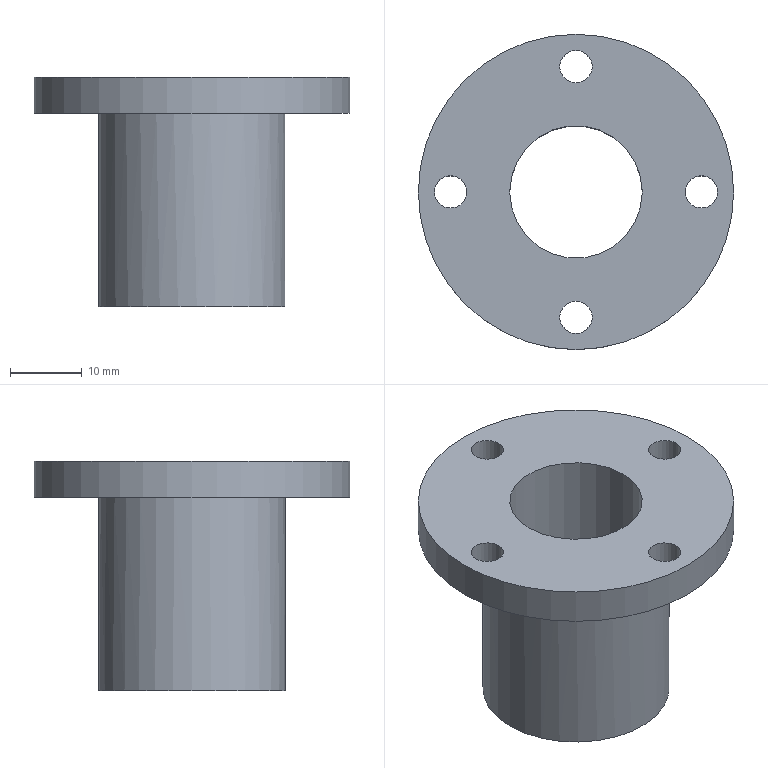Part | STEP file | YBQDJ-YL-17 | 1 solid | 10 faces | box 44 x 44 x 32 mm | volume 13018 mm3 | cylinder 7 | plane 3 | commonest cylinder face diameters 4.5 x4 18.5 x1 26 x1 44 x1
STEP:
#1=CARTESIAN_POINT('',(0.,0.,0.));
#2=DIRECTION('',(0.,0.,1.));
#3=DIRECTION('',(1.,0.,0.));
#4=AXIS2_PLACEMENT_3D('',#1,#2,#3);
#5=CARTESIAN_POINT('',(306.5,-210.25,170.));
#6=VERTEX_POINT('',#5);
#7=CARTESIAN_POINT('',(306.5,-212.5,170.));
#8=DIRECTION('',(0.,0.,-1.));
#9=DIRECTION('',(0.,1.,0.));
#10=AXIS2_PLACEMENT_3D('',#7,#8,#9);
#11=CIRCLE('',#10,2.25);
#12=CARTESIAN_POINT('',(306.5,-212.5,170.));
#13=DIRECTION('',(0.,0.,-1.));
#14=DIRECTION('',(1.,0.,0.));
#15=AXIS2_PLACEMENT_3D('',#12,#13,#14);
#16=CYLINDRICAL_SURFACE('',#15,2.25);
#17=CARTESIAN_POINT('',(4.712,0.));
#18=DIRECTION('',(1.,0.));
#19=VECTOR('',#18,1.);
#20=LINE('',#17,#19);
#21=(GEOMETRIC_REPRESENTATION_CONTEXT(2)PARAMETRIC_REPRESENTATION_CONTEXT()REPRESENTATION_CONTEXT('',''));
#22=DEFINITIONAL_REPRESENTATION('',(#20),#21);
#23=PCURVE('',#16,#22);
#24=CARTESIAN_POINT('',(306.5,-195.,170.));
#25=DIRECTION('',(0.,0.,1.));
#26=DIRECTION('',(0.,-1.,0.));
#27=AXIS2_PLACEMENT_3D('',#24,#25,#26);
#28=PLANE('',#27);
#29=CARTESIAN_POINT('',(15.25,0.));
#30=CARTESIAN_POINT('',(15.25,3.897));
#31=CARTESIAN_POINT('',(18.625,1.949));
#32=CARTESIAN_POINT('',(22.,0.));
#33=CARTESIAN_POINT('',(18.625,-1.949));
#34=CARTESIAN_POINT('',(15.25,-3.897));
#35=CARTESIAN_POINT('',(15.25,0.));
#36=(BOUNDED_CURVE()B_SPLINE_CURVE(2,(#29,#30,#31,#32,#33,#34,#35),.UNSPECIFIED.,.T.,.F.)B_SPLINE_CURVE_WITH_KNOTS((1,2,2,2,2,1),(-2.094,0.,2.094,4.189,6.283,8.378),.UNSPECIFIED.)CURVE()GEOMETRIC_REPRESENTATION_ITEM()RATIONAL_B_SPLINE_CURVE((1.,0.5,1.,0.5,1.,0.5,1.))REPRESENTATION_ITEM(''));
#37=(GEOMETRIC_REPRESENTATION_CONTEXT(2)PARAMETRIC_REPRESENTATION_CONTEXT()REPRESENTATION_CONTEXT('',''));
#38=DEFINITIONAL_REPRESENTATION('',(#36),#37);
#39=PCURVE('',#28,#38);
#40=SURFACE_CURVE('',#11,(#23,#39),.PCURVE_S1.);
#41=EDGE_CURVE('',#6,#6,#40,.T.);
#42=ORIENTED_EDGE('',*,*,#41,.T.);
#43=CARTESIAN_POINT('',(306.5,-210.25,165.));
#44=VERTEX_POINT('',#43);
#45=CARTESIAN_POINT('',(306.5,-210.25,170.));
#46=CARTESIAN_POINT('',(306.5,-210.25,165.));
#47=B_SPLINE_CURVE_WITH_KNOTS('',1,(#45,#46),.UNSPECIFIED.,.F.,.F.,(2,2),(0.,5.),.PIECEWISE_BEZIER_KNOTS.);
#48=CARTESIAN_POINT('',(10.996,0.));
#49=DIRECTION('',(0.,1.));
#50=VECTOR('',#49,1.);
#51=LINE('',#48,#50);
#52=(GEOMETRIC_REPRESENTATION_CONTEXT(2)PARAMETRIC_REPRESENTATION_CONTEXT()REPRESENTATION_CONTEXT('',''));
#53=DEFINITIONAL_REPRESENTATION('',(#51),#52);
#54=PCURVE('',#16,#53);
#55=CARTESIAN_POINT('',(4.712,0.));
#56=DIRECTION('',(0.,1.));
#57=VECTOR('',#56,1.);
#58=LINE('',#55,#57);
#59=(GEOMETRIC_REPRESENTATION_CONTEXT(2)PARAMETRIC_REPRESENTATION_CONTEXT()REPRESENTATION_CONTEXT('',''));
#60=DEFINITIONAL_REPRESENTATION('',(#58),#59);
#61=PCURVE('',#16,#60);
#62=SEAM_CURVE('',#47,(#54,#61),.PCURVE_S1.);
#63=EDGE_CURVE('',#6,#44,#62,.T.);
#64=ORIENTED_EDGE('',*,*,#63,.T.);
#65=CARTESIAN_POINT('',(306.5,-212.5,165.));
#66=DIRECTION('',(0.,0.,1.));
#67=DIRECTION('',(0.,1.,0.));
#68=AXIS2_PLACEMENT_3D('',#65,#66,#67);
#69=CIRCLE('',#68,2.25);
#70=CARTESIAN_POINT('',(10.996,5.));
#71=DIRECTION('',(-1.,0.));
#72=VECTOR('',#71,1.);
#73=LINE('',#70,#72);
#74=(GEOMETRIC_REPRESENTATION_CONTEXT(2)PARAMETRIC_REPRESENTATION_CONTEXT()REPRESENTATION_CONTEXT('',''));
#75=DEFINITIONAL_REPRESENTATION('',(#73),#74);
#76=PCURVE('',#16,#75);
#77=CARTESIAN_POINT('',(306.5,-195.,165.));
#78=DIRECTION('',(0.,0.,1.));
#79=DIRECTION('',(0.,-1.,0.));
#80=AXIS2_PLACEMENT_3D('',#77,#78,#79);
#81=PLANE('',#80);
#82=CARTESIAN_POINT('',(17.5,0.));
#83=DIRECTION('',(-1.,0.));
#84=AXIS2_PLACEMENT_2D('',#82,#83);
#85=CIRCLE('',#84,2.25);
#86=(GEOMETRIC_REPRESENTATION_CONTEXT(2)PARAMETRIC_REPRESENTATION_CONTEXT()REPRESENTATION_CONTEXT('',''));
#87=DEFINITIONAL_REPRESENTATION('',(#85),#86);
#88=PCURVE('',#81,#87);
#89=SURFACE_CURVE('',#69,(#76,#88),.PCURVE_S1.);
#90=EDGE_CURVE('',#44,#44,#89,.T.);
#91=ORIENTED_EDGE('',*,*,#90,.T.);
#92=ORIENTED_EDGE('',*,*,#63,.F.);
#93=EDGE_LOOP('',(#42,#64,#91,#92));
#94=FACE_BOUND('',#93,.F.);
#95=ADVANCED_FACE('',(#94),#16,.F.);
#96=CARTESIAN_POINT('',(297.25,-195.,138.));
#97=VERTEX_POINT('',#96);
#98=CARTESIAN_POINT('',(315.75,-195.,138.));
#99=VERTEX_POINT('',#98);
#100=CARTESIAN_POINT('',(306.5,-195.,138.));
#101=DIRECTION('',(0.,0.,1.));
#102=DIRECTION('',(-1.,0.,0.));
#103=AXIS2_PLACEMENT_3D('',#100,#101,#102);
#104=CIRCLE('',#103,9.25);
#105=CARTESIAN_POINT('',(306.5,-195.,138.));
#106=DIRECTION('',(0.,0.,-1.));
#107=DIRECTION('',(0.,1.,0.));
#108=AXIS2_PLACEMENT_3D('',#105,#106,#107);
#109=PLANE('',#108);
#110=CARTESIAN_POINT('',(0.,-9.25));
#111=CARTESIAN_POINT('',(-16.021,-9.25));
#112=CARTESIAN_POINT('',(-8.011,4.625));
#113=CARTESIAN_POINT('',(0.,18.5));
#114=CARTESIAN_POINT('',(8.011,4.625));
#115=CARTESIAN_POINT('',(16.021,-9.25));
#116=CARTESIAN_POINT('',(0.,-9.25));
#117=(BOUNDED_CURVE()B_SPLINE_CURVE(2,(#110,#111,#112,#113,#114,#115,#116),.UNSPECIFIED.,.T.,.F.)B_SPLINE_CURVE_WITH_KNOTS((1,2,2,2,2,1),(-2.094,0.,2.094,4.189,6.283,8.378),.UNSPECIFIED.)CURVE()GEOMETRIC_REPRESENTATION_ITEM()RATIONAL_B_SPLINE_CURVE((1.,0.5,1.,0.5,1.,0.5,1.))REPRESENTATION_ITEM(''));
#118=(GEOMETRIC_REPRESENTATION_CONTEXT(2)PARAMETRIC_REPRESENTATION_CONTEXT()REPRESENTATION_CONTEXT('',''));
#119=DEFINITIONAL_REPRESENTATION('',(#117),#118);
#120=PCURVE('',#109,#119);
#121=CARTESIAN_POINT('',(306.5,-195.,142.));
#122=DIRECTION('',(0.,0.,1.));
#123=DIRECTION('',(0.,-1.,0.));
#124=AXIS2_PLACEMENT_3D('',#121,#122,#123);
#125=CYLINDRICAL_SURFACE('',#124,9.25);
#126=CARTESIAN_POINT('',(4.712,-4.));
#127=DIRECTION('',(1.,0.));
#128=VECTOR('',#127,1.);
#129=LINE('',#126,#128);
#130=(GEOMETRIC_REPRESENTATION_CONTEXT(2)PARAMETRIC_REPRESENTATION_CONTEXT()REPRESENTATION_CONTEXT('',''));
#131=DEFINITIONAL_REPRESENTATION('',(#129),#130);
#132=PCURVE('',#125,#131);
#133=SURFACE_CURVE('',#104,(#120,#132),.PCURVE_S1.);
#134=EDGE_CURVE('',#97,#99,#133,.T.);
#135=ORIENTED_EDGE('',*,*,#134,.T.);
#136=CARTESIAN_POINT('',(306.5,-195.,138.));
#137=DIRECTION('',(0.,0.,1.));
#138=DIRECTION('',(-1.,0.,0.));
#139=AXIS2_PLACEMENT_3D('',#136,#137,#138);
#140=CIRCLE('',#139,9.25);
#141=CARTESIAN_POINT('',(0.,-9.25));
#142=CARTESIAN_POINT('',(-16.021,-9.25));
#143=CARTESIAN_POINT('',(-8.011,4.625));
#144=CARTESIAN_POINT('',(0.,18.5));
#145=CARTESIAN_POINT('',(8.011,4.625));
#146=CARTESIAN_POINT('',(16.021,-9.25));
#147=CARTESIAN_POINT('',(0.,-9.25));
#148=(BOUNDED_CURVE()B_SPLINE_CURVE(2,(#141,#142,#143,#144,#145,#146,#147),.UNSPECIFIED.,.T.,.F.)B_SPLINE_CURVE_WITH_KNOTS((1,2,2,2,2,1),(-2.094,0.,2.094,4.189,6.283,8.378),.UNSPECIFIED.)CURVE()GEOMETRIC_REPRESENTATION_ITEM()RATIONAL_B_SPLINE_CURVE((1.,0.5,1.,0.5,1.,0.5,1.))REPRESENTATION_ITEM(''));
#149=(GEOMETRIC_REPRESENTATION_CONTEXT(2)PARAMETRIC_REPRESENTATION_CONTEXT()REPRESENTATION_CONTEXT('',''));
#150=DEFINITIONAL_REPRESENTATION('',(#148),#149);
#151=PCURVE('',#109,#150);
#152=CARTESIAN_POINT('',(-1.571,-4.));
#153=DIRECTION('',(1.,0.));
#154=VECTOR('',#153,1.);
#155=LINE('',#152,#154);
#156=(GEOMETRIC_REPRESENTATION_CONTEXT(2)PARAMETRIC_REPRESENTATION_CONTEXT()REPRESENTATION_CONTEXT('',''));
#157=DEFINITIONAL_REPRESENTATION('',(#155),#156);
#158=PCURVE('',#125,#157);
#159=SURFACE_CURVE('',#140,(#151,#158),.PCURVE_S1.);
#160=EDGE_CURVE('',#99,#97,#159,.T.);
#161=ORIENTED_EDGE('',*,*,#160,.T.);
#162=EDGE_LOOP('',(#135,#161));
#163=FACE_BOUND('',#162,.T.);
#164=CARTESIAN_POINT('',(293.5,-195.,138.));
#165=VERTEX_POINT('',#164);
#166=CARTESIAN_POINT('',(306.5,-195.,138.));
#167=DIRECTION('',(0.,0.,-1.));
#168=DIRECTION('',(-1.,0.,0.));
#169=AXIS2_PLACEMENT_3D('',#166,#167,#168);
#170=CIRCLE('',#169,13.);
#171=CARTESIAN_POINT('',(0.,0.));
#172=DIRECTION('',(0.,-1.));
#173=AXIS2_PLACEMENT_2D('',#171,#172);
#174=CIRCLE('',#173,13.);
#175=(GEOMETRIC_REPRESENTATION_CONTEXT(2)PARAMETRIC_REPRESENTATION_CONTEXT()REPRESENTATION_CONTEXT('',''));
#176=DEFINITIONAL_REPRESENTATION('',(#174),#175);
#177=PCURVE('',#109,#176);
#178=CARTESIAN_POINT('',(306.5,-195.,165.));
#179=DIRECTION('',(0.,0.,-1.));
#180=DIRECTION('',(0.,1.,0.));
#181=AXIS2_PLACEMENT_3D('',#178,#179,#180);
#182=CYLINDRICAL_SURFACE('',#181,13.);
#183=CARTESIAN_POINT('',(4.712,27.));
#184=DIRECTION('',(1.,0.));
#185=VECTOR('',#184,1.);
#186=LINE('',#183,#185);
#187=(GEOMETRIC_REPRESENTATION_CONTEXT(2)PARAMETRIC_REPRESENTATION_CONTEXT()REPRESENTATION_CONTEXT('',''));
#188=DEFINITIONAL_REPRESENTATION('',(#186),#187);
#189=PCURVE('',#182,#188);
#190=SURFACE_CURVE('',#170,(#177,#189),.PCURVE_S1.);
#191=EDGE_CURVE('',#165,#165,#190,.T.);
#192=ORIENTED_EDGE('',*,*,#191,.T.);
#193=EDGE_LOOP('',(#192));
#194=FACE_BOUND('',#193,.T.);
#195=ADVANCED_FACE('',(#163,#194),#109,.T.);
#196=CARTESIAN_POINT('',(291.25,-195.,170.));
#197=VERTEX_POINT('',#196);
#198=CARTESIAN_POINT('',(289.,-195.,170.));
#199=DIRECTION('',(0.,0.,1.));
#200=DIRECTION('',(1.,0.,0.));
#201=AXIS2_PLACEMENT_3D('',#198,#199,#200);
#202=CIRCLE('',#201,2.25);
#203=CARTESIAN_POINT('',(289.,-195.,170.));
#204=DIRECTION('',(0.,0.,-1.));
#205=DIRECTION('',(0.,1.,0.));
#206=AXIS2_PLACEMENT_3D('',#203,#204,#205);
#207=CYLINDRICAL_SURFACE('',#206,2.25);
#208=CARTESIAN_POINT('',(7.854,0.));
#209=DIRECTION('',(-1.,0.));
#210=VECTOR('',#209,1.);
#211=LINE('',#208,#210);
#212=(GEOMETRIC_REPRESENTATION_CONTEXT(2)PARAMETRIC_REPRESENTATION_CONTEXT()REPRESENTATION_CONTEXT('',''));
#213=DEFINITIONAL_REPRESENTATION('',(#211),#212);
#214=PCURVE('',#207,#213);
#215=CARTESIAN_POINT('',(0.,-17.5));
#216=DIRECTION('',(0.,1.));
#217=AXIS2_PLACEMENT_2D('',#215,#216);
#218=CIRCLE('',#217,2.25);
#219=(GEOMETRIC_REPRESENTATION_CONTEXT(2)PARAMETRIC_REPRESENTATION_CONTEXT()REPRESENTATION_CONTEXT('',''));
#220=DEFINITIONAL_REPRESENTATION('',(#218),#219);
#221=PCURVE('',#28,#220);
#222=SURFACE_CURVE('',#202,(#214,#221),.PCURVE_S1.);
#223=EDGE_CURVE('',#197,#197,#222,.T.);
#224=ORIENTED_EDGE('',*,*,#223,.F.);
#225=CARTESIAN_POINT('',(291.25,-195.,165.));
#226=VERTEX_POINT('',#225);
#227=CARTESIAN_POINT('',(291.25,-195.,170.));
#228=CARTESIAN_POINT('',(291.25,-195.,165.));
#229=B_SPLINE_CURVE_WITH_KNOTS('',1,(#227,#228),.UNSPECIFIED.,.F.,.F.,(2,2),(0.,5.),.PIECEWISE_BEZIER_KNOTS.);
#230=CARTESIAN_POINT('',(7.854,0.));
#231=DIRECTION('',(0.,1.));
#232=VECTOR('',#231,1.);
#233=LINE('',#230,#232);
#234=(GEOMETRIC_REPRESENTATION_CONTEXT(2)PARAMETRIC_REPRESENTATION_CONTEXT()REPRESENTATION_CONTEXT('',''));
#235=DEFINITIONAL_REPRESENTATION('',(#233),#234);
#236=PCURVE('',#207,#235);
#237=CARTESIAN_POINT('',(1.571,0.));
#238=DIRECTION('',(0.,1.));
#239=VECTOR('',#238,1.);
#240=LINE('',#237,#239);
#241=(GEOMETRIC_REPRESENTATION_CONTEXT(2)PARAMETRIC_REPRESENTATION_CONTEXT()REPRESENTATION_CONTEXT('',''));
#242=DEFINITIONAL_REPRESENTATION('',(#240),#241);
#243=PCURVE('',#207,#242);
#244=SEAM_CURVE('',#229,(#236,#243),.PCURVE_S1.);
#245=EDGE_CURVE('',#197,#226,#244,.T.);
#246=ORIENTED_EDGE('',*,*,#245,.T.);
#247=CARTESIAN_POINT('',(289.,-195.,165.));
#248=DIRECTION('',(0.,0.,1.));
#249=DIRECTION('',(1.,0.,0.));
#250=AXIS2_PLACEMENT_3D('',#247,#248,#249);
#251=CIRCLE('',#250,2.25);
#252=CARTESIAN_POINT('',(7.854,5.));
#253=DIRECTION('',(-1.,0.));
#254=VECTOR('',#253,1.);
#255=LINE('',#252,#254);
#256=(GEOMETRIC_REPRESENTATION_CONTEXT(2)PARAMETRIC_REPRESENTATION_CONTEXT()REPRESENTATION_CONTEXT('',''));
#257=DEFINITIONAL_REPRESENTATION('',(#255),#256);
#258=PCURVE('',#207,#257);
#259=CARTESIAN_POINT('',(0.,-17.5));
#260=DIRECTION('',(0.,1.));
#261=AXIS2_PLACEMENT_2D('',#259,#260);
#262=CIRCLE('',#261,2.25);
#263=(GEOMETRIC_REPRESENTATION_CONTEXT(2)PARAMETRIC_REPRESENTATION_CONTEXT()REPRESENTATION_CONTEXT('',''));
#264=DEFINITIONAL_REPRESENTATION('',(#262),#263);
#265=PCURVE('',#81,#264);
#266=SURFACE_CURVE('',#251,(#258,#265),.PCURVE_S1.);
#267=EDGE_CURVE('',#226,#226,#266,.T.);
#268=ORIENTED_EDGE('',*,*,#267,.T.);
#269=ORIENTED_EDGE('',*,*,#245,.F.);
#270=EDGE_LOOP('',(#224,#246,#268,#269));
#271=FACE_BOUND('',#270,.F.);
#272=ADVANCED_FACE('',(#271),#207,.F.);
#273=CARTESIAN_POINT('',(321.75,-195.,170.));
#274=VERTEX_POINT('',#273);
#275=CARTESIAN_POINT('',(324.,-195.,170.));
#276=DIRECTION('',(0.,0.,-1.));
#277=DIRECTION('',(-1.,0.,0.));
#278=AXIS2_PLACEMENT_3D('',#275,#276,#277);
#279=CIRCLE('',#278,2.25);
#280=CARTESIAN_POINT('',(324.,-195.,170.));
#281=DIRECTION('',(0.,0.,-1.));
#282=DIRECTION('',(0.,1.,0.));
#283=AXIS2_PLACEMENT_3D('',#280,#281,#282);
#284=CYLINDRICAL_SURFACE('',#283,2.25);
#285=CARTESIAN_POINT('',(4.712,0.));
#286=DIRECTION('',(1.,0.));
#287=VECTOR('',#286,1.);
#288=LINE('',#285,#287);
#289=(GEOMETRIC_REPRESENTATION_CONTEXT(2)PARAMETRIC_REPRESENTATION_CONTEXT()REPRESENTATION_CONTEXT('',''));
#290=DEFINITIONAL_REPRESENTATION('',(#288),#289);
#291=PCURVE('',#284,#290);
#292=CARTESIAN_POINT('',(0.,15.25));
#293=CARTESIAN_POINT('',(-3.897,15.25));
#294=CARTESIAN_POINT('',(-1.949,18.625));
#295=CARTESIAN_POINT('',(0.,22.));
#296=CARTESIAN_POINT('',(1.949,18.625));
#297=CARTESIAN_POINT('',(3.897,15.25));
#298=CARTESIAN_POINT('',(0.,15.25));
#299=(BOUNDED_CURVE()B_SPLINE_CURVE(2,(#292,#293,#294,#295,#296,#297,#298),.UNSPECIFIED.,.T.,.F.)B_SPLINE_CURVE_WITH_KNOTS((1,2,2,2,2,1),(-2.094,0.,2.094,4.189,6.283,8.378),.UNSPECIFIED.)CURVE()GEOMETRIC_REPRESENTATION_ITEM()RATIONAL_B_SPLINE_CURVE((1.,0.5,1.,0.5,1.,0.5,1.))REPRESENTATION_ITEM(''));
#300=(GEOMETRIC_REPRESENTATION_CONTEXT(2)PARAMETRIC_REPRESENTATION_CONTEXT()REPRESENTATION_CONTEXT('',''));
#301=DEFINITIONAL_REPRESENTATION('',(#299),#300);
#302=PCURVE('',#28,#301);
#303=SURFACE_CURVE('',#279,(#291,#302),.PCURVE_S1.);
#304=EDGE_CURVE('',#274,#274,#303,.T.);
#305=ORIENTED_EDGE('',*,*,#304,.T.);
#306=CARTESIAN_POINT('',(321.75,-195.,165.));
#307=VERTEX_POINT('',#306);
#308=CARTESIAN_POINT('',(321.75,-195.,170.));
#309=CARTESIAN_POINT('',(321.75,-195.,165.));
#310=B_SPLINE_CURVE_WITH_KNOTS('',1,(#308,#309),.UNSPECIFIED.,.F.,.F.,(2,2),(0.,5.),.PIECEWISE_BEZIER_KNOTS.);
#311=CARTESIAN_POINT('',(10.996,0.));
#312=DIRECTION('',(0.,1.));
#313=VECTOR('',#312,1.);
#314=LINE('',#311,#313);
#315=(GEOMETRIC_REPRESENTATION_CONTEXT(2)PARAMETRIC_REPRESENTATION_CONTEXT()REPRESENTATION_CONTEXT('',''));
#316=DEFINITIONAL_REPRESENTATION('',(#314),#315);
#317=PCURVE('',#284,#316);
#318=CARTESIAN_POINT('',(4.712,0.));
#319=DIRECTION('',(0.,1.));
#320=VECTOR('',#319,1.);
#321=LINE('',#318,#320);
#322=(GEOMETRIC_REPRESENTATION_CONTEXT(2)PARAMETRIC_REPRESENTATION_CONTEXT()REPRESENTATION_CONTEXT('',''));
#323=DEFINITIONAL_REPRESENTATION('',(#321),#322);
#324=PCURVE('',#284,#323);
#325=SEAM_CURVE('',#310,(#317,#324),.PCURVE_S1.);
#326=EDGE_CURVE('',#274,#307,#325,.T.);
#327=ORIENTED_EDGE('',*,*,#326,.T.);
#328=CARTESIAN_POINT('',(324.,-195.,165.));
#329=DIRECTION('',(0.,0.,-1.));
#330=DIRECTION('',(-1.,0.,0.));
#331=AXIS2_PLACEMENT_3D('',#328,#329,#330);
#332=CIRCLE('',#331,2.25);
#333=CARTESIAN_POINT('',(4.712,5.));
#334=DIRECTION('',(1.,0.));
#335=VECTOR('',#334,1.);
#336=LINE('',#333,#335);
#337=(GEOMETRIC_REPRESENTATION_CONTEXT(2)PARAMETRIC_REPRESENTATION_CONTEXT()REPRESENTATION_CONTEXT('',''));
#338=DEFINITIONAL_REPRESENTATION('',(#336),#337);
#339=PCURVE('',#284,#338);
#340=CARTESIAN_POINT('',(0.,15.25));
#341=CARTESIAN_POINT('',(-3.897,15.25));
#342=CARTESIAN_POINT('',(-1.949,18.625));
#343=CARTESIAN_POINT('',(0.,22.));
#344=CARTESIAN_POINT('',(1.949,18.625));
#345=CARTESIAN_POINT('',(3.897,15.25));
#346=CARTESIAN_POINT('',(0.,15.25));
#347=(BOUNDED_CURVE()B_SPLINE_CURVE(2,(#340,#341,#342,#343,#344,#345,#346),.UNSPECIFIED.,.T.,.F.)B_SPLINE_CURVE_WITH_KNOTS((1,2,2,2,2,1),(-2.094,0.,2.094,4.189,6.283,8.378),.UNSPECIFIED.)CURVE()GEOMETRIC_REPRESENTATION_ITEM()RATIONAL_B_SPLINE_CURVE((1.,0.5,1.,0.5,1.,0.5,1.))REPRESENTATION_ITEM(''));
#348=(GEOMETRIC_REPRESENTATION_CONTEXT(2)PARAMETRIC_REPRESENTATION_CONTEXT()REPRESENTATION_CONTEXT('',''));
#349=DEFINITIONAL_REPRESENTATION('',(#347),#348);
#350=PCURVE('',#81,#349);
#351=SURFACE_CURVE('',#332,(#339,#350),.PCURVE_S1.);
#352=EDGE_CURVE('',#307,#307,#351,.T.);
#353=ORIENTED_EDGE('',*,*,#352,.F.);
#354=ORIENTED_EDGE('',*,*,#326,.F.);
#355=EDGE_LOOP('',(#305,#327,#353,#354));
#356=FACE_BOUND('',#355,.F.);
#357=ADVANCED_FACE('',(#356),#284,.F.);
#358=CARTESIAN_POINT('',(328.5,-195.,165.));
#359=VERTEX_POINT('',#358);
#360=CARTESIAN_POINT('',(306.5,-195.,165.));
#361=DIRECTION('',(0.,0.,1.));
#362=DIRECTION('',(1.,0.,0.));
#363=AXIS2_PLACEMENT_3D('',#360,#361,#362);
#364=CIRCLE('',#363,22.);
#365=CARTESIAN_POINT('',(306.5,-195.,170.));
#366=DIRECTION('',(0.,0.,-1.));
#367=DIRECTION('',(0.,1.,0.));
#368=AXIS2_PLACEMENT_3D('',#365,#366,#367);
#369=CYLINDRICAL_SURFACE('',#368,22.);
#370=CARTESIAN_POINT('',(7.854,5.));
#371=DIRECTION('',(-1.,0.));
#372=VECTOR('',#371,1.);
#373=LINE('',#370,#372);
#374=(GEOMETRIC_REPRESENTATION_CONTEXT(2)PARAMETRIC_REPRESENTATION_CONTEXT()REPRESENTATION_CONTEXT('',''));
#375=DEFINITIONAL_REPRESENTATION('',(#373),#374);
#376=PCURVE('',#369,#375);
#377=CARTESIAN_POINT('',(0.,0.));
#378=DIRECTION('',(0.,1.));
#379=AXIS2_PLACEMENT_2D('',#377,#378);
#380=CIRCLE('',#379,22.);
#381=(GEOMETRIC_REPRESENTATION_CONTEXT(2)PARAMETRIC_REPRESENTATION_CONTEXT()REPRESENTATION_CONTEXT('',''));
#382=DEFINITIONAL_REPRESENTATION('',(#380),#381);
#383=PCURVE('',#81,#382);
#384=SURFACE_CURVE('',#364,(#376,#383),.PCURVE_S1.);
#385=EDGE_CURVE('',#359,#359,#384,.T.);
#386=ORIENTED_EDGE('',*,*,#385,.T.);
#387=CARTESIAN_POINT('',(328.5,-195.,170.));
#388=VERTEX_POINT('',#387);
#389=CARTESIAN_POINT('',(328.5,-195.,170.));
#390=CARTESIAN_POINT('',(328.5,-195.,165.));
#391=B_SPLINE_CURVE_WITH_KNOTS('',1,(#389,#390),.UNSPECIFIED.,.F.,.F.,(2,2),(0.,5.),.PIECEWISE_BEZIER_KNOTS.);
#392=CARTESIAN_POINT('',(1.571,0.));
#393=DIRECTION('',(0.,1.));
#394=VECTOR('',#393,1.);
#395=LINE('',#392,#394);
#396=(GEOMETRIC_REPRESENTATION_CONTEXT(2)PARAMETRIC_REPRESENTATION_CONTEXT()REPRESENTATION_CONTEXT('',''));
#397=DEFINITIONAL_REPRESENTATION('',(#395),#396);
#398=PCURVE('',#369,#397);
#399=CARTESIAN_POINT('',(7.854,0.));
#400=DIRECTION('',(0.,1.));
#401=VECTOR('',#400,1.);
#402=LINE('',#399,#401);
#403=(GEOMETRIC_REPRESENTATION_CONTEXT(2)PARAMETRIC_REPRESENTATION_CONTEXT()REPRESENTATION_CONTEXT('',''));
#404=DEFINITIONAL_REPRESENTATION('',(#402),#403);
#405=PCURVE('',#369,#404);
#406=SEAM_CURVE('',#391,(#398,#405),.PCURVE_S1.);
#407=EDGE_CURVE('',#388,#359,#406,.T.);
#408=ORIENTED_EDGE('',*,*,#407,.F.);
#409=CARTESIAN_POINT('',(306.5,-195.,170.));
#410=DIRECTION('',(0.,0.,1.));
#411=DIRECTION('',(1.,0.,0.));
#412=AXIS2_PLACEMENT_3D('',#409,#410,#411);
#413=CIRCLE('',#412,22.);
#414=CARTESIAN_POINT('',(7.854,0.));
#415=DIRECTION('',(-1.,0.));
#416=VECTOR('',#415,1.);
#417=LINE('',#414,#416);
#418=(GEOMETRIC_REPRESENTATION_CONTEXT(2)PARAMETRIC_REPRESENTATION_CONTEXT()REPRESENTATION_CONTEXT('',''));
#419=DEFINITIONAL_REPRESENTATION('',(#417),#418);
#420=PCURVE('',#369,#419);
#421=CARTESIAN_POINT('',(0.,0.));
#422=DIRECTION('',(0.,1.));
#423=AXIS2_PLACEMENT_2D('',#421,#422);
#424=CIRCLE('',#423,22.);
#425=(GEOMETRIC_REPRESENTATION_CONTEXT(2)PARAMETRIC_REPRESENTATION_CONTEXT()REPRESENTATION_CONTEXT('',''));
#426=DEFINITIONAL_REPRESENTATION('',(#424),#425);
#427=PCURVE('',#28,#426);
#428=SURFACE_CURVE('',#413,(#420,#427),.PCURVE_S1.);
#429=EDGE_CURVE('',#388,#388,#428,.T.);
#430=ORIENTED_EDGE('',*,*,#429,.F.);
#431=ORIENTED_EDGE('',*,*,#407,.T.);
#432=EDGE_LOOP('',(#386,#408,#430,#431));
#433=FACE_BOUND('',#432,.T.);
#434=ADVANCED_FACE('',(#433),#369,.T.);
#435=CARTESIAN_POINT('',(319.5,-195.,165.));
#436=VERTEX_POINT('',#435);
#437=CARTESIAN_POINT('',(293.5,-195.,165.));
#438=VERTEX_POINT('',#437);
#439=CARTESIAN_POINT('',(306.5,-195.,165.));
#440=DIRECTION('',(0.,0.,-1.));
#441=DIRECTION('',(1.,0.,0.));
#442=AXIS2_PLACEMENT_3D('',#439,#440,#441);
#443=CIRCLE('',#442,13.);
#444=CARTESIAN_POINT('',(7.854,0.));
#445=DIRECTION('',(1.,0.));
#446=VECTOR('',#445,1.);
#447=LINE('',#444,#446);
#448=(GEOMETRIC_REPRESENTATION_CONTEXT(2)PARAMETRIC_REPRESENTATION_CONTEXT()REPRESENTATION_CONTEXT('',''));
#449=DEFINITIONAL_REPRESENTATION('',(#447),#448);
#450=PCURVE('',#182,#449);
#451=CARTESIAN_POINT('',(0.,13.));
#452=CARTESIAN_POINT('',(22.517,13.));
#453=CARTESIAN_POINT('',(11.258,-6.5));
#454=CARTESIAN_POINT('',(0.,-26.));
#455=CARTESIAN_POINT('',(-11.258,-6.5));
#456=CARTESIAN_POINT('',(-22.517,13.));
#457=CARTESIAN_POINT('',(0.,13.));
#458=(BOUNDED_CURVE()B_SPLINE_CURVE(2,(#451,#452,#453,#454,#455,#456,#457),.UNSPECIFIED.,.T.,.F.)B_SPLINE_CURVE_WITH_KNOTS((1,2,2,2,2,1),(-2.094,0.,2.094,4.189,6.283,8.378),.UNSPECIFIED.)CURVE()GEOMETRIC_REPRESENTATION_ITEM()RATIONAL_B_SPLINE_CURVE((1.,0.5,1.,0.5,1.,0.5,1.))REPRESENTATION_ITEM(''));
#459=(GEOMETRIC_REPRESENTATION_CONTEXT(2)PARAMETRIC_REPRESENTATION_CONTEXT()REPRESENTATION_CONTEXT('',''));
#460=DEFINITIONAL_REPRESENTATION('',(#458),#459);
#461=PCURVE('',#81,#460);
#462=SURFACE_CURVE('',#443,(#450,#461),.PCURVE_S1.);
#463=EDGE_CURVE('',#436,#438,#462,.T.);
#464=ORIENTED_EDGE('',*,*,#463,.T.);
#465=CARTESIAN_POINT('',(293.5,-195.,165.));
#466=CARTESIAN_POINT('',(293.5,-195.,138.));
#467=B_SPLINE_CURVE_WITH_KNOTS('',1,(#465,#466),.UNSPECIFIED.,.F.,.F.,(2,2),(0.,27.),.PIECEWISE_BEZIER_KNOTS.);
#468=CARTESIAN_POINT('',(10.996,0.));
#469=DIRECTION('',(0.,1.));
#470=VECTOR('',#469,1.);
#471=LINE('',#468,#470);
#472=(GEOMETRIC_REPRESENTATION_CONTEXT(2)PARAMETRIC_REPRESENTATION_CONTEXT()REPRESENTATION_CONTEXT('',''));
#473=DEFINITIONAL_REPRESENTATION('',(#471),#472);
#474=PCURVE('',#182,#473);
#475=CARTESIAN_POINT('',(4.712,0.));
#476=DIRECTION('',(0.,1.));
#477=VECTOR('',#476,1.);
#478=LINE('',#475,#477);
#479=(GEOMETRIC_REPRESENTATION_CONTEXT(2)PARAMETRIC_REPRESENTATION_CONTEXT()REPRESENTATION_CONTEXT('',''));
#480=DEFINITIONAL_REPRESENTATION('',(#478),#479);
#481=PCURVE('',#182,#480);
#482=SEAM_CURVE('',#467,(#474,#481),.PCURVE_S1.);
#483=EDGE_CURVE('',#438,#165,#482,.T.);
#484=ORIENTED_EDGE('',*,*,#483,.T.);
#485=ORIENTED_EDGE('',*,*,#191,.F.);
#486=ORIENTED_EDGE('',*,*,#483,.F.);
#487=CARTESIAN_POINT('',(306.5,-195.,165.));
#488=DIRECTION('',(0.,0.,-1.));
#489=DIRECTION('',(1.,0.,0.));
#490=AXIS2_PLACEMENT_3D('',#487,#488,#489);
#491=CIRCLE('',#490,13.);
#492=CARTESIAN_POINT('',(1.571,0.));
#493=DIRECTION('',(1.,0.));
#494=VECTOR('',#493,1.);
#495=LINE('',#492,#494);
#496=(GEOMETRIC_REPRESENTATION_CONTEXT(2)PARAMETRIC_REPRESENTATION_CONTEXT()REPRESENTATION_CONTEXT('',''));
#497=DEFINITIONAL_REPRESENTATION('',(#495),#496);
#498=PCURVE('',#182,#497);
#499=CARTESIAN_POINT('',(0.,13.));
#500=CARTESIAN_POINT('',(22.517,13.));
#501=CARTESIAN_POINT('',(11.258,-6.5));
#502=CARTESIAN_POINT('',(0.,-26.));
#503=CARTESIAN_POINT('',(-11.258,-6.5));
#504=CARTESIAN_POINT('',(-22.517,13.));
#505=CARTESIAN_POINT('',(0.,13.));
#506=(BOUNDED_CURVE()B_SPLINE_CURVE(2,(#499,#500,#501,#502,#503,#504,#505),.UNSPECIFIED.,.T.,.F.)B_SPLINE_CURVE_WITH_KNOTS((1,2,2,2,2,1),(-2.094,0.,2.094,4.189,6.283,8.378),.UNSPECIFIED.)CURVE()GEOMETRIC_REPRESENTATION_ITEM()RATIONAL_B_SPLINE_CURVE((1.,0.5,1.,0.5,1.,0.5,1.))REPRESENTATION_ITEM(''));
#507=(GEOMETRIC_REPRESENTATION_CONTEXT(2)PARAMETRIC_REPRESENTATION_CONTEXT()REPRESENTATION_CONTEXT('',''));
#508=DEFINITIONAL_REPRESENTATION('',(#506),#507);
#509=PCURVE('',#81,#508);
#510=SURFACE_CURVE('',#491,(#498,#509),.PCURVE_S1.);
#511=EDGE_CURVE('',#438,#436,#510,.T.);
#512=ORIENTED_EDGE('',*,*,#511,.T.);
#513=EDGE_LOOP('',(#464,#484,#485,#486,#512));
#514=FACE_BOUND('',#513,.T.);
#515=ADVANCED_FACE('',(#514),#182,.T.);
#516=CARTESIAN_POINT('',(306.5,-179.75,165.));
#517=VERTEX_POINT('',#516);
#518=CARTESIAN_POINT('',(306.5,-177.5,165.));
#519=DIRECTION('',(0.,0.,1.));
#520=DIRECTION('',(0.,-1.,0.));
#521=AXIS2_PLACEMENT_3D('',#518,#519,#520);
#522=CIRCLE('',#521,2.25);
#523=CARTESIAN_POINT('',(-17.5,0.));
#524=DIRECTION('',(1.,0.));
#525=AXIS2_PLACEMENT_2D('',#523,#524);
#526=CIRCLE('',#525,2.25);
#527=(GEOMETRIC_REPRESENTATION_CONTEXT(2)PARAMETRIC_REPRESENTATION_CONTEXT()REPRESENTATION_CONTEXT('',''));
#528=DEFINITIONAL_REPRESENTATION('',(#526),#527);
#529=PCURVE('',#81,#528);
#530=CARTESIAN_POINT('',(306.5,-177.5,170.));
#531=DIRECTION('',(0.,0.,-1.));
#532=DIRECTION('',(1.,0.,0.));
#533=AXIS2_PLACEMENT_3D('',#530,#531,#532);
#534=CYLINDRICAL_SURFACE('',#533,2.25);
#535=CARTESIAN_POINT('',(7.854,5.));
#536=DIRECTION('',(-1.,0.));
#537=VECTOR('',#536,1.);
#538=LINE('',#535,#537);
#539=(GEOMETRIC_REPRESENTATION_CONTEXT(2)PARAMETRIC_REPRESENTATION_CONTEXT()REPRESENTATION_CONTEXT('',''));
#540=DEFINITIONAL_REPRESENTATION('',(#538),#539);
#541=PCURVE('',#534,#540);
#542=SURFACE_CURVE('',#522,(#529,#541),.PCURVE_S1.);
#543=EDGE_CURVE('',#517,#517,#542,.T.);
#544=ORIENTED_EDGE('',*,*,#543,.T.);
#545=EDGE_LOOP('',(#544));
#546=FACE_BOUND('',#545,.T.);
#547=ORIENTED_EDGE('',*,*,#90,.T.);
#548=EDGE_LOOP('',(#547));
#549=FACE_BOUND('',#548,.T.);
#550=ORIENTED_EDGE('',*,*,#463,.F.);
#551=ORIENTED_EDGE('',*,*,#511,.F.);
#552=EDGE_LOOP('',(#550,#551));
#553=FACE_BOUND('',#552,.T.);
#554=ORIENTED_EDGE('',*,*,#385,.F.);
#555=EDGE_LOOP('',(#554));
#556=FACE_BOUND('',#555,.T.);
#557=ORIENTED_EDGE('',*,*,#352,.F.);
#558=EDGE_LOOP('',(#557));
#559=FACE_BOUND('',#558,.T.);
#560=ORIENTED_EDGE('',*,*,#267,.T.);
#561=EDGE_LOOP('',(#560));
#562=FACE_BOUND('',#561,.T.);
#563=ADVANCED_FACE('',(#546,#549,#553,#556,#559,#562),#81,.F.);
#564=ORIENTED_EDGE('',*,*,#134,.T.);
#565=CARTESIAN_POINT('',(315.75,-195.,170.));
#566=VERTEX_POINT('',#565);
#567=CARTESIAN_POINT('',(315.75,-195.,138.));
#568=CARTESIAN_POINT('',(315.75,-195.,170.));
#569=B_SPLINE_CURVE_WITH_KNOTS('',1,(#567,#568),.UNSPECIFIED.,.F.,.F.,(2,2),(-4.,28.),.PIECEWISE_BEZIER_KNOTS.);
#570=CARTESIAN_POINT('',(7.854,0.));
#571=DIRECTION('',(0.,1.));
#572=VECTOR('',#571,1.);
#573=LINE('',#570,#572);
#574=(GEOMETRIC_REPRESENTATION_CONTEXT(2)PARAMETRIC_REPRESENTATION_CONTEXT()REPRESENTATION_CONTEXT('',''));
#575=DEFINITIONAL_REPRESENTATION('',(#573),#574);
#576=PCURVE('',#125,#575);
#577=CARTESIAN_POINT('',(1.571,0.));
#578=DIRECTION('',(0.,1.));
#579=VECTOR('',#578,1.);
#580=LINE('',#577,#579);
#581=(GEOMETRIC_REPRESENTATION_CONTEXT(2)PARAMETRIC_REPRESENTATION_CONTEXT()REPRESENTATION_CONTEXT('',''));
#582=DEFINITIONAL_REPRESENTATION('',(#580),#581);
#583=PCURVE('',#125,#582);
#584=SEAM_CURVE('',#569,(#576,#583),.PCURVE_S1.);
#585=EDGE_CURVE('',#99,#566,#584,.T.);
#586=ORIENTED_EDGE('',*,*,#585,.T.);
#587=CARTESIAN_POINT('',(306.5,-195.,170.));
#588=DIRECTION('',(0.,0.,1.));
#589=DIRECTION('',(1.,0.,0.));
#590=AXIS2_PLACEMENT_3D('',#587,#588,#589);
#591=CIRCLE('',#590,9.25);
#592=CARTESIAN_POINT('',(1.571,28.));
#593=DIRECTION('',(1.,0.));
#594=VECTOR('',#593,1.);
#595=LINE('',#592,#594);
#596=(GEOMETRIC_REPRESENTATION_CONTEXT(2)PARAMETRIC_REPRESENTATION_CONTEXT()REPRESENTATION_CONTEXT('',''));
#597=DEFINITIONAL_REPRESENTATION('',(#595),#596);
#598=PCURVE('',#125,#597);
#599=CARTESIAN_POINT('',(0.,0.));
#600=DIRECTION('',(0.,1.));
#601=AXIS2_PLACEMENT_2D('',#599,#600);
#602=CIRCLE('',#601,9.25);
#603=(GEOMETRIC_REPRESENTATION_CONTEXT(2)PARAMETRIC_REPRESENTATION_CONTEXT()REPRESENTATION_CONTEXT('',''));
#604=DEFINITIONAL_REPRESENTATION('',(#602),#603);
#605=PCURVE('',#28,#604);
#606=SURFACE_CURVE('',#591,(#598,#605),.PCURVE_S1.);
#607=EDGE_CURVE('',#566,#566,#606,.T.);
#608=ORIENTED_EDGE('',*,*,#607,.F.);
#609=ORIENTED_EDGE('',*,*,#585,.F.);
#610=ORIENTED_EDGE('',*,*,#160,.T.);
#611=EDGE_LOOP('',(#564,#586,#608,#609,#610));
#612=FACE_BOUND('',#611,.F.);
#613=ADVANCED_FACE('',(#612),#125,.F.);
#614=CARTESIAN_POINT('',(306.5,-179.75,170.));
#615=VERTEX_POINT('',#614);
#616=CARTESIAN_POINT('',(306.5,-177.5,170.));
#617=DIRECTION('',(0.,0.,-1.));
#618=DIRECTION('',(0.,-1.,0.));
#619=AXIS2_PLACEMENT_3D('',#616,#617,#618);
#620=CIRCLE('',#619,2.25);
#621=CARTESIAN_POINT('',(-15.25,0.));
#622=CARTESIAN_POINT('',(-15.25,-3.897));
#623=CARTESIAN_POINT('',(-18.625,-1.949));
#624=CARTESIAN_POINT('',(-22.,0.));
#625=CARTESIAN_POINT('',(-18.625,1.949));
#626=CARTESIAN_POINT('',(-15.25,3.897));
#627=CARTESIAN_POINT('',(-15.25,0.));
#628=(BOUNDED_CURVE()B_SPLINE_CURVE(2,(#621,#622,#623,#624,#625,#626,#627),.UNSPECIFIED.,.T.,.F.)B_SPLINE_CURVE_WITH_KNOTS((1,2,2,2,2,1),(-2.094,0.,2.094,4.189,6.283,8.378),.UNSPECIFIED.)CURVE()GEOMETRIC_REPRESENTATION_ITEM()RATIONAL_B_SPLINE_CURVE((1.,0.5,1.,0.5,1.,0.5,1.))REPRESENTATION_ITEM(''));
#629=(GEOMETRIC_REPRESENTATION_CONTEXT(2)PARAMETRIC_REPRESENTATION_CONTEXT()REPRESENTATION_CONTEXT('',''));
#630=DEFINITIONAL_REPRESENTATION('',(#628),#629);
#631=PCURVE('',#28,#630);
#632=CARTESIAN_POINT('',(1.571,0.));
#633=DIRECTION('',(1.,0.));
#634=VECTOR('',#633,1.);
#635=LINE('',#632,#634);
#636=(GEOMETRIC_REPRESENTATION_CONTEXT(2)PARAMETRIC_REPRESENTATION_CONTEXT()REPRESENTATION_CONTEXT('',''));
#637=DEFINITIONAL_REPRESENTATION('',(#635),#636);
#638=PCURVE('',#534,#637);
#639=SURFACE_CURVE('',#620,(#631,#638),.PCURVE_S1.);
#640=EDGE_CURVE('',#615,#615,#639,.T.);
#641=ORIENTED_EDGE('',*,*,#640,.T.);
#642=EDGE_LOOP('',(#641));
#643=FACE_BOUND('',#642,.T.);
#644=ORIENTED_EDGE('',*,*,#41,.T.);
#645=EDGE_LOOP('',(#644));
#646=FACE_BOUND('',#645,.T.);
#647=ORIENTED_EDGE('',*,*,#607,.F.);
#648=EDGE_LOOP('',(#647));
#649=FACE_BOUND('',#648,.T.);
#650=ORIENTED_EDGE('',*,*,#429,.T.);
#651=EDGE_LOOP('',(#650));
#652=FACE_BOUND('',#651,.T.);
#653=ORIENTED_EDGE('',*,*,#304,.T.);
#654=EDGE_LOOP('',(#653));
#655=FACE_BOUND('',#654,.T.);
#656=ORIENTED_EDGE('',*,*,#223,.F.);
#657=EDGE_LOOP('',(#656));
#658=FACE_BOUND('',#657,.T.);
#659=ADVANCED_FACE('',(#643,#646,#649,#652,#655,#658),#28,.T.);
#660=ORIENTED_EDGE('',*,*,#640,.T.);
#661=CARTESIAN_POINT('',(306.5,-179.75,170.));
#662=CARTESIAN_POINT('',(306.5,-179.75,165.));
#663=B_SPLINE_CURVE_WITH_KNOTS('',1,(#661,#662),.UNSPECIFIED.,.F.,.F.,(2,2),(0.,5.),.PIECEWISE_BEZIER_KNOTS.);
#664=CARTESIAN_POINT('',(7.854,0.));
#665=DIRECTION('',(0.,1.));
#666=VECTOR('',#665,1.);
#667=LINE('',#664,#666);
#668=(GEOMETRIC_REPRESENTATION_CONTEXT(2)PARAMETRIC_REPRESENTATION_CONTEXT()REPRESENTATION_CONTEXT('',''));
#669=DEFINITIONAL_REPRESENTATION('',(#667),#668);
#670=PCURVE('',#534,#669);
#671=CARTESIAN_POINT('',(1.571,0.));
#672=DIRECTION('',(0.,1.));
#673=VECTOR('',#672,1.);
#674=LINE('',#671,#673);
#675=(GEOMETRIC_REPRESENTATION_CONTEXT(2)PARAMETRIC_REPRESENTATION_CONTEXT()REPRESENTATION_CONTEXT('',''));
#676=DEFINITIONAL_REPRESENTATION('',(#674),#675);
#677=PCURVE('',#534,#676);
#678=SEAM_CURVE('',#663,(#670,#677),.PCURVE_S1.);
#679=EDGE_CURVE('',#615,#517,#678,.T.);
#680=ORIENTED_EDGE('',*,*,#679,.T.);
#681=ORIENTED_EDGE('',*,*,#543,.T.);
#682=ORIENTED_EDGE('',*,*,#679,.F.);
#683=EDGE_LOOP('',(#660,#680,#681,#682));
#684=FACE_BOUND('',#683,.F.);
#685=ADVANCED_FACE('',(#684),#534,.F.);
#686=CLOSED_SHELL('',(#95,#195,#272,#357,#434,#515,#563,#613,#659,#685));
#687=MANIFOLD_SOLID_BREP('',#686);
#688=(LENGTH_UNIT()NAMED_UNIT(*)SI_UNIT(.MILLI.,.METRE.));
#689=UNCERTAINTY_MEASURE_WITH_UNIT(LENGTH_MEASURE(0.000005),#688,'','');
#690=(NAMED_UNIT(*)PLANE_ANGLE_UNIT()SI_UNIT($,.RADIAN.));
#691=(NAMED_UNIT(*)SI_UNIT($,.STERADIAN.)SOLID_ANGLE_UNIT());
#692=(GEOMETRIC_REPRESENTATION_CONTEXT(3)GLOBAL_UNCERTAINTY_ASSIGNED_CONTEXT((#689))GLOBAL_UNIT_ASSIGNED_CONTEXT((#688,#690,#691))REPRESENTATION_CONTEXT('',''));
#693=ADVANCED_BREP_SHAPE_REPRESENTATION('',(#4,#687),#692);